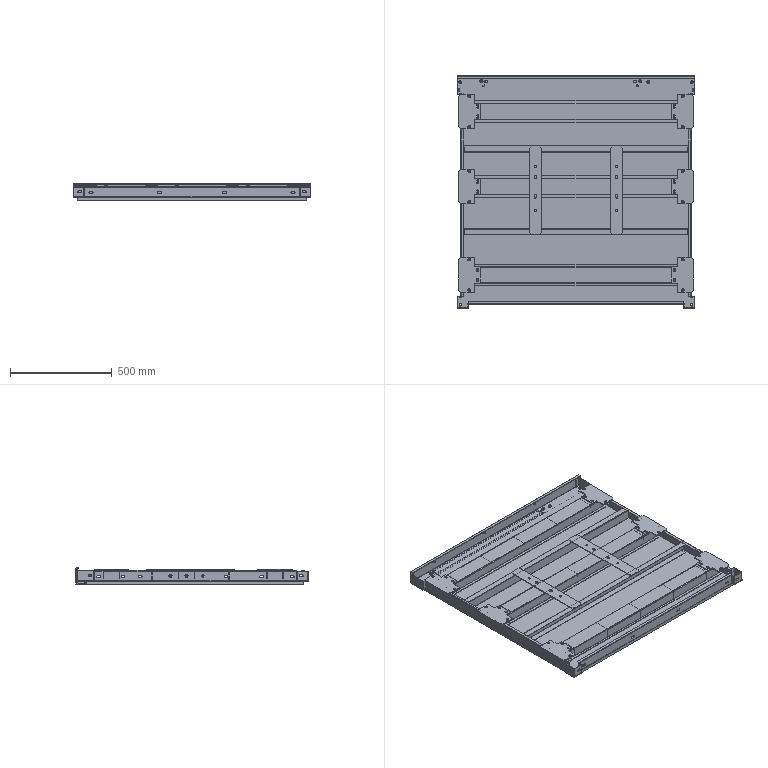Part | SolidWorks | features ReferencePattern 3, MirrorCompFeat 1 | 77 solids | 2214 faces | box 1171 x 1143 x 83 mm | volume 26404069 mm3 | plane 1507 | cylinder 509 | cone 168 | spline 30 | commonest cylinder face diameters 10 x80 6.917 x56 10.45 x56 10.77 x56 0.4 x44 6.4 x36